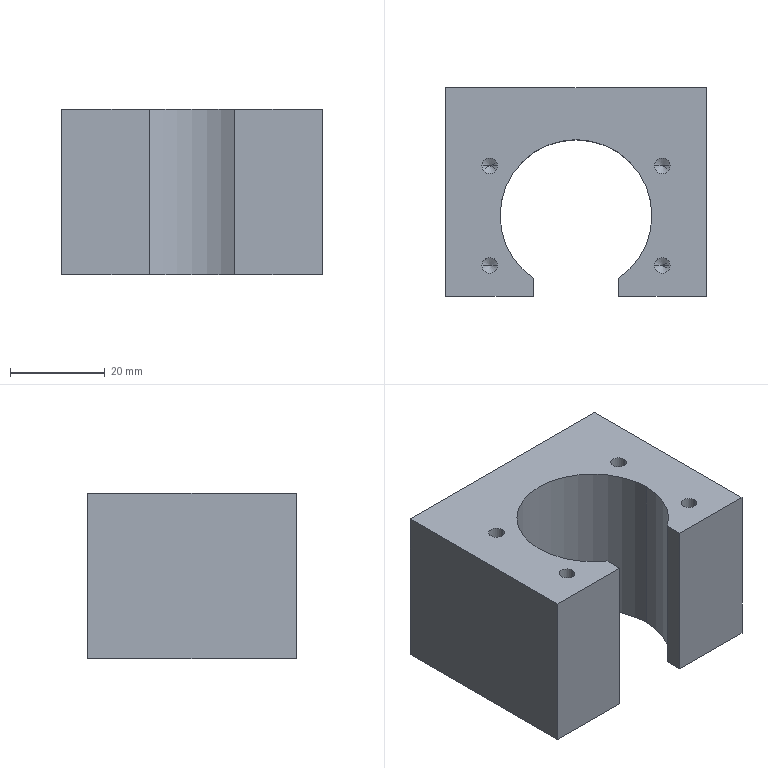Part | SolidWorks | features HoleWzd 2, 3DProfileFeature 1, Extrusion 1 | 1 solid | 52 faces | box 55 x 44 x 35 mm | volume 54034 mm3 | cone 24 | cylinder 19 | plane 9 | commonest cylinder face diameters 3.3 x8 5 x8 32 x3
STEP:
#1=CARTESIAN_POINT('',(-20.5,26.475,8.));
#2=VERTEX_POINT('',#1);
#3=CARTESIAN_POINT('',(-20.5,26.475,13.));
#4=VERTEX_POINT('',#3);
#5=CARTESIAN_POINT('',(-20.5,26.475,10.5));
#6=DIRECTION('',(0.,1.,0.));
#7=DIRECTION('',(0.,0.,1.));
#8=AXIS2_PLACEMENT_3D('',#5,#6,#7);
#9=CIRCLE('',#8,2.5);
#10=EDGE_CURVE('',#2,#4,#9,.T.);
#11=ORIENTED_EDGE('',*,*,#10,.F.);
#12=CARTESIAN_POINT('',(-20.5,27.,7.475));
#13=VERTEX_POINT('',#12);
#14=CARTESIAN_POINT('',(-20.5,27.,7.475));
#15=DIRECTION('',(0.,0.7071,-0.7071));
#16=VECTOR('',#15,1000.);
#17=LINE('',#14,#16);
#18=EDGE_CURVE('',#2,#13,#17,.T.);
#19=ORIENTED_EDGE('',*,*,#18,.T.);
#20=CARTESIAN_POINT('',(-20.5,27.,13.525));
#21=VERTEX_POINT('',#20);
#22=CARTESIAN_POINT('',(-20.5,27.,10.5));
#23=DIRECTION('',(0.,1.,0.));
#24=DIRECTION('',(0.,0.,1.));
#25=AXIS2_PLACEMENT_3D('',#22,#23,#24);
#26=CIRCLE('',#25,3.025);
#27=EDGE_CURVE('',#13,#21,#26,.T.);
#28=ORIENTED_EDGE('',*,*,#27,.T.);
#29=CARTESIAN_POINT('',(-20.5,27.,13.525));
#30=DIRECTION('',(0.,0.7071,0.7071));
#31=VECTOR('',#30,1000.);
#32=LINE('',#29,#31);
#33=EDGE_CURVE('',#4,#21,#32,.T.);
#34=ORIENTED_EDGE('',*,*,#33,.F.);
#35=EDGE_LOOP('',(#11,#19,#28,#34));
#36=FACE_OUTER_BOUND('',#35,.T.);
#37=CARTESIAN_POINT('',(-20.5,27.,10.5));
#38=DIRECTION('',(0.,1.,0.));
#39=DIRECTION('',(0.,0.,1.));
#40=AXIS2_PLACEMENT_3D('',#37,#38,#39);
#41=CONICAL_SURFACE('',#40,3.025,0.7854);
#42=ADVANCED_FACE('',(#36),#41,.F.);
#43=CARTESIAN_POINT('',(-20.5,15.,8.));
#44=VERTEX_POINT('',#43);
#45=CARTESIAN_POINT('',(-20.5,15.,13.));
#46=VERTEX_POINT('',#45);
#47=CARTESIAN_POINT('',(-20.5,15.,10.5));
#48=DIRECTION('',(0.,1.,0.));
#49=DIRECTION('',(0.,0.,1.));
#50=AXIS2_PLACEMENT_3D('',#47,#48,#49);
#51=CIRCLE('',#50,2.5);
#52=EDGE_CURVE('',#44,#46,#51,.T.);
#53=ORIENTED_EDGE('',*,*,#52,.F.);
#54=CARTESIAN_POINT('',(-20.5,27.,8.));
#55=DIRECTION('',(0.,1.,0.));
#56=VECTOR('',#55,1000.);
#57=LINE('',#54,#56);
#58=EDGE_CURVE('',#44,#2,#57,.T.);
#59=ORIENTED_EDGE('',*,*,#58,.T.);
#60=ORIENTED_EDGE('',*,*,#10,.T.);
#61=CARTESIAN_POINT('',(-20.5,27.,13.));
#62=DIRECTION('',(0.,1.,0.));
#63=VECTOR('',#62,1000.);
#64=LINE('',#61,#63);
#65=EDGE_CURVE('',#46,#4,#64,.T.);
#66=ORIENTED_EDGE('',*,*,#65,.F.);
#67=EDGE_LOOP('',(#53,#59,#60,#66));
#68=FACE_OUTER_BOUND('',#67,.T.);
#69=CARTESIAN_POINT('',(-20.5,27.,10.5));
#70=DIRECTION('',(0.,1.,0.));
#71=DIRECTION('',(0.,0.,1.));
#72=AXIS2_PLACEMENT_3D('',#69,#70,#71);
#73=CYLINDRICAL_SURFACE('',#72,2.5);
#74=ADVANCED_FACE('',(#68),#73,.F.);
#75=CARTESIAN_POINT('',(-20.5,13.498,10.5));
#76=VERTEX_POINT('',#75);
#77=CARTESIAN_POINT('',(-20.5,15.,13.));
#78=DIRECTION('',(0.,0.515,0.8572));
#79=VECTOR('',#78,1000.);
#80=LINE('',#77,#79);
#81=EDGE_CURVE('',#76,#46,#80,.T.);
#82=ORIENTED_EDGE('',*,*,#81,.F.);
#83=CARTESIAN_POINT('',(-20.5,15.,8.));
#84=DIRECTION('',(0.,0.515,-0.8572));
#85=VECTOR('',#84,1000.);
#86=LINE('',#83,#85);
#87=EDGE_CURVE('',#76,#44,#86,.T.);
#88=ORIENTED_EDGE('',*,*,#87,.T.);
#89=ORIENTED_EDGE('',*,*,#52,.T.);
#90=EDGE_LOOP('',(#82,#88,#89));
#91=FACE_OUTER_BOUND('',#90,.T.);
#92=CARTESIAN_POINT('',(-20.5,15.,10.5));
#93=DIRECTION('',(0.,1.,0.));
#94=DIRECTION('',(0.,0.,1.));
#95=AXIS2_PLACEMENT_3D('',#92,#93,#94);
#96=CONICAL_SURFACE('',#95,2.5,1.03);
#97=ADVANCED_FACE('',(#91),#96,.F.);
#98=CARTESIAN_POINT('',(-20.5,26.475,-13.));
#99=VERTEX_POINT('',#98);
#100=CARTESIAN_POINT('',(-20.5,26.475,-8.));
#101=VERTEX_POINT('',#100);
#102=CARTESIAN_POINT('',(-20.5,26.475,-10.5));
#103=DIRECTION('',(0.,1.,0.));
#104=DIRECTION('',(0.,0.,1.));
#105=AXIS2_PLACEMENT_3D('',#102,#103,#104);
#106=CIRCLE('',#105,2.5);
#107=EDGE_CURVE('',#99,#101,#106,.T.);
#108=ORIENTED_EDGE('',*,*,#107,.F.);
#109=CARTESIAN_POINT('',(-20.5,27.,-13.525));
#110=VERTEX_POINT('',#109);
#111=CARTESIAN_POINT('',(-20.5,27.,-13.525));
#112=DIRECTION('',(0.,0.7071,-0.7071));
#113=VECTOR('',#112,1000.);
#114=LINE('',#111,#113);
#115=EDGE_CURVE('',#99,#110,#114,.T.);
#116=ORIENTED_EDGE('',*,*,#115,.T.);
#117=CARTESIAN_POINT('',(-20.5,27.,-7.475));
#118=VERTEX_POINT('',#117);
#119=CARTESIAN_POINT('',(-20.5,27.,-10.5));
#120=DIRECTION('',(0.,1.,0.));
#121=DIRECTION('',(0.,0.,1.));
#122=AXIS2_PLACEMENT_3D('',#119,#120,#121);
#123=CIRCLE('',#122,3.025);
#124=EDGE_CURVE('',#110,#118,#123,.T.);
#125=ORIENTED_EDGE('',*,*,#124,.T.);
#126=CARTESIAN_POINT('',(-20.5,27.,-7.475));
#127=DIRECTION('',(0.,0.7071,0.7071));
#128=VECTOR('',#127,1000.);
#129=LINE('',#126,#128);
#130=EDGE_CURVE('',#101,#118,#129,.T.);
#131=ORIENTED_EDGE('',*,*,#130,.F.);
#132=EDGE_LOOP('',(#108,#116,#125,#131));
#133=FACE_OUTER_BOUND('',#132,.T.);
#134=CARTESIAN_POINT('',(-20.5,27.,-10.5));
#135=DIRECTION('',(0.,1.,0.));
#136=DIRECTION('',(0.,0.,1.));
#137=AXIS2_PLACEMENT_3D('',#134,#135,#136);
#138=CONICAL_SURFACE('',#137,3.025,0.7854);
#139=ADVANCED_FACE('',(#133),#138,.F.);
#140=CARTESIAN_POINT('',(-20.5,15.,-13.));
#141=VERTEX_POINT('',#140);
#142=CARTESIAN_POINT('',(-20.5,15.,-8.));
#143=VERTEX_POINT('',#142);
#144=CARTESIAN_POINT('',(-20.5,15.,-10.5));
#145=DIRECTION('',(0.,1.,0.));
#146=DIRECTION('',(0.,0.,1.));
#147=AXIS2_PLACEMENT_3D('',#144,#145,#146);
#148=CIRCLE('',#147,2.5);
#149=EDGE_CURVE('',#141,#143,#148,.T.);
#150=ORIENTED_EDGE('',*,*,#149,.F.);
#151=CARTESIAN_POINT('',(-20.5,27.,-13.));
#152=DIRECTION('',(0.,1.,0.));
#153=VECTOR('',#152,1000.);
#154=LINE('',#151,#153);
#155=EDGE_CURVE('',#141,#99,#154,.T.);
#156=ORIENTED_EDGE('',*,*,#155,.T.);
#157=ORIENTED_EDGE('',*,*,#107,.T.);
#158=CARTESIAN_POINT('',(-20.5,27.,-8.));
#159=DIRECTION('',(0.,1.,0.));
#160=VECTOR('',#159,1000.);
#161=LINE('',#158,#160);
#162=EDGE_CURVE('',#143,#101,#161,.T.);
#163=ORIENTED_EDGE('',*,*,#162,.F.);
#164=EDGE_LOOP('',(#150,#156,#157,#163));
#165=FACE_OUTER_BOUND('',#164,.T.);
#166=CARTESIAN_POINT('',(-20.5,27.,-10.5));
#167=DIRECTION('',(0.,1.,0.));
#168=DIRECTION('',(0.,0.,1.));
#169=AXIS2_PLACEMENT_3D('',#166,#167,#168);
#170=CYLINDRICAL_SURFACE('',#169,2.5);
#171=ADVANCED_FACE('',(#165),#170,.F.);
#172=CARTESIAN_POINT('',(-20.5,13.498,-10.5));
#173=VERTEX_POINT('',#172);
#174=CARTESIAN_POINT('',(-20.5,15.,-8.));
#175=DIRECTION('',(0.,0.515,0.8572));
#176=VECTOR('',#175,1000.);
#177=LINE('',#174,#176);
#178=EDGE_CURVE('',#173,#143,#177,.T.);
#179=ORIENTED_EDGE('',*,*,#178,.F.);
#180=CARTESIAN_POINT('',(-20.5,15.,-13.));
#181=DIRECTION('',(0.,0.515,-0.8572));
#182=VECTOR('',#181,1000.);
#183=LINE('',#180,#182);
#184=EDGE_CURVE('',#173,#141,#183,.T.);
#185=ORIENTED_EDGE('',*,*,#184,.T.);
#186=ORIENTED_EDGE('',*,*,#149,.T.);
#187=EDGE_LOOP('',(#179,#185,#186));
#188=FACE_OUTER_BOUND('',#187,.T.);
#189=CARTESIAN_POINT('',(-20.5,15.,-10.5));
#190=DIRECTION('',(0.,1.,0.));
#191=DIRECTION('',(0.,0.,1.));
#192=AXIS2_PLACEMENT_3D('',#189,#190,#191);
#193=CONICAL_SURFACE('',#192,2.5,1.03);
#194=ADVANCED_FACE('',(#188),#193,.F.);
#195=CARTESIAN_POINT('',(20.5,26.475,-13.));
#196=VERTEX_POINT('',#195);
#197=CARTESIAN_POINT('',(20.5,26.475,-8.));
#198=VERTEX_POINT('',#197);
#199=CARTESIAN_POINT('',(20.5,26.475,-10.5));
#200=DIRECTION('',(0.,1.,0.));
#201=DIRECTION('',(0.,0.,1.));
#202=AXIS2_PLACEMENT_3D('',#199,#200,#201);
#203=CIRCLE('',#202,2.5);
#204=EDGE_CURVE('',#196,#198,#203,.T.);
#205=ORIENTED_EDGE('',*,*,#204,.F.);
#206=CARTESIAN_POINT('',(20.5,27.,-13.525));
#207=VERTEX_POINT('',#206);
#208=CARTESIAN_POINT('',(20.5,27.,-13.525));
#209=DIRECTION('',(0.,0.7071,-0.7071));
#210=VECTOR('',#209,1000.);
#211=LINE('',#208,#210);
#212=EDGE_CURVE('',#196,#207,#211,.T.);
#213=ORIENTED_EDGE('',*,*,#212,.T.);
#214=CARTESIAN_POINT('',(20.5,27.,-7.475));
#215=VERTEX_POINT('',#214);
#216=CARTESIAN_POINT('',(20.5,27.,-10.5));
#217=DIRECTION('',(0.,1.,0.));
#218=DIRECTION('',(0.,0.,1.));
#219=AXIS2_PLACEMENT_3D('',#216,#217,#218);
#220=CIRCLE('',#219,3.025);
#221=EDGE_CURVE('',#207,#215,#220,.T.);
#222=ORIENTED_EDGE('',*,*,#221,.T.);
#223=CARTESIAN_POINT('',(20.5,27.,-7.475));
#224=DIRECTION('',(0.,0.7071,0.7071));
#225=VECTOR('',#224,1000.);
#226=LINE('',#223,#225);
#227=EDGE_CURVE('',#198,#215,#226,.T.);
#228=ORIENTED_EDGE('',*,*,#227,.F.);
#229=EDGE_LOOP('',(#205,#213,#222,#228));
#230=FACE_OUTER_BOUND('',#229,.T.);
#231=CARTESIAN_POINT('',(20.5,27.,-10.5));
#232=DIRECTION('',(0.,1.,0.));
#233=DIRECTION('',(0.,0.,1.));
#234=AXIS2_PLACEMENT_3D('',#231,#232,#233);
#235=CONICAL_SURFACE('',#234,3.025,0.7854);
#236=ADVANCED_FACE('',(#230),#235,.F.);
#237=CARTESIAN_POINT('',(20.5,15.,-13.));
#238=VERTEX_POINT('',#237);
#239=CARTESIAN_POINT('',(20.5,15.,-8.));
#240=VERTEX_POINT('',#239);
#241=CARTESIAN_POINT('',(20.5,15.,-10.5));
#242=DIRECTION('',(0.,1.,0.));
#243=DIRECTION('',(0.,0.,1.));
#244=AXIS2_PLACEMENT_3D('',#241,#242,#243);
#245=CIRCLE('',#244,2.5);
#246=EDGE_CURVE('',#238,#240,#245,.T.);
#247=ORIENTED_EDGE('',*,*,#246,.F.);
#248=CARTESIAN_POINT('',(20.5,27.,-13.));
#249=DIRECTION('',(0.,1.,0.));
#250=VECTOR('',#249,1000.);
#251=LINE('',#248,#250);
#252=EDGE_CURVE('',#238,#196,#251,.T.);
#253=ORIENTED_EDGE('',*,*,#252,.T.);
#254=ORIENTED_EDGE('',*,*,#204,.T.);
#255=CARTESIAN_POINT('',(20.5,27.,-8.));
#256=DIRECTION('',(0.,1.,0.));
#257=VECTOR('',#256,1000.);
#258=LINE('',#255,#257);
#259=EDGE_CURVE('',#240,#198,#258,.T.);
#260=ORIENTED_EDGE('',*,*,#259,.F.);
#261=EDGE_LOOP('',(#247,#253,#254,#260));
#262=FACE_OUTER_BOUND('',#261,.T.);
#263=CARTESIAN_POINT('',(20.5,27.,-10.5));
#264=DIRECTION('',(0.,1.,0.));
#265=DIRECTION('',(0.,0.,1.));
#266=AXIS2_PLACEMENT_3D('',#263,#264,#265);
#267=CYLINDRICAL_SURFACE('',#266,2.5);
#268=ADVANCED_FACE('',(#262),#267,.F.);
#269=CARTESIAN_POINT('',(20.5,13.498,-10.5));
#270=VERTEX_POINT('',#269);
#271=CARTESIAN_POINT('',(20.5,15.,-8.));
#272=DIRECTION('',(0.,0.515,0.8572));
#273=VECTOR('',#272,1000.);
#274=LINE('',#271,#273);
#275=EDGE_CURVE('',#270,#240,#274,.T.);
#276=ORIENTED_EDGE('',*,*,#275,.F.);
#277=CARTESIAN_POINT('',(20.5,15.,-13.));
#278=DIRECTION('',(0.,0.515,-0.8572));
#279=VECTOR('',#278,1000.);
#280=LINE('',#277,#279);
#281=EDGE_CURVE('',#270,#238,#280,.T.);
#282=ORIENTED_EDGE('',*,*,#281,.T.);
#283=ORIENTED_EDGE('',*,*,#246,.T.);
#284=EDGE_LOOP('',(#276,#282,#283));
#285=FACE_OUTER_BOUND('',#284,.T.);
#286=CARTESIAN_POINT('',(20.5,15.,-10.5));
#287=DIRECTION('',(0.,1.,0.));
#288=DIRECTION('',(0.,0.,1.));
#289=AXIS2_PLACEMENT_3D('',#286,#287,#288);
#290=CONICAL_SURFACE('',#289,2.5,1.03);
#291=ADVANCED_FACE('',(#285),#290,.F.);
#292=CARTESIAN_POINT('',(20.5,26.475,8.));
#293=VERTEX_POINT('',#292);
#294=CARTESIAN_POINT('',(20.5,26.475,13.));
#295=VERTEX_POINT('',#294);
#296=CARTESIAN_POINT('',(20.5,26.475,10.5));
#297=DIRECTION('',(0.,1.,0.));
#298=DIRECTION('',(0.,0.,1.));
#299=AXIS2_PLACEMENT_3D('',#296,#297,#298);
#300=CIRCLE('',#299,2.5);
#301=EDGE_CURVE('',#293,#295,#300,.T.);
#302=ORIENTED_EDGE('',*,*,#301,.F.);
#303=CARTESIAN_POINT('',(20.5,27.,7.475));
#304=VERTEX_POINT('',#303);
#305=CARTESIAN_POINT('',(20.5,27.,7.475));
#306=DIRECTION('',(0.,0.7071,-0.7071));
#307=VECTOR('',#306,1000.);
#308=LINE('',#305,#307);
#309=EDGE_CURVE('',#293,#304,#308,.T.);
#310=ORIENTED_EDGE('',*,*,#309,.T.);
#311=CARTESIAN_POINT('',(20.5,27.,13.525));
#312=VERTEX_POINT('',#311);
#313=CARTESIAN_POINT('',(20.5,27.,10.5));
#314=DIRECTION('',(0.,1.,0.));
#315=DIRECTION('',(0.,0.,1.));
#316=AXIS2_PLACEMENT_3D('',#313,#314,#315);
#317=CIRCLE('',#316,3.025);
#318=EDGE_CURVE('',#304,#312,#317,.T.);
#319=ORIENTED_EDGE('',*,*,#318,.T.);
#320=CARTESIAN_POINT('',(20.5,27.,13.525));
#321=DIRECTION('',(0.,0.7071,0.7071));
#322=VECTOR('',#321,1000.);
#323=LINE('',#320,#322);
#324=EDGE_CURVE('',#295,#312,#323,.T.);
#325=ORIENTED_EDGE('',*,*,#324,.F.);
#326=EDGE_LOOP('',(#302,#310,#319,#325));
#327=FACE_OUTER_BOUND('',#326,.T.);
#328=CARTESIAN_POINT('',(20.5,27.,10.5));
#329=DIRECTION('',(0.,1.,0.));
#330=DIRECTION('',(0.,0.,1.));
#331=AXIS2_PLACEMENT_3D('',#328,#329,#330);
#332=CONICAL_SURFACE('',#331,3.025,0.7854);
#333=ADVANCED_FACE('',(#327),#332,.F.);
#334=CARTESIAN_POINT('',(20.5,15.,8.));
#335=VERTEX_POINT('',#334);
#336=CARTESIAN_POINT('',(20.5,15.,13.));
#337=VERTEX_POINT('',#336);
#338=CARTESIAN_POINT('',(20.5,15.,10.5));
#339=DIRECTION('',(0.,1.,0.));
#340=DIRECTION('',(0.,0.,1.));
#341=AXIS2_PLACEMENT_3D('',#338,#339,#340);
#342=CIRCLE('',#341,2.5);
#343=EDGE_CURVE('',#335,#337,#342,.T.);
#344=ORIENTED_EDGE('',*,*,#343,.F.);
#345=CARTESIAN_POINT('',(20.5,27.,8.));
#346=DIRECTION('',(0.,1.,0.));
#347=VECTOR('',#346,1000.);
#348=LINE('',#345,#347);
#349=EDGE_CURVE('',#335,#293,#348,.T.);
#350=ORIENTED_EDGE('',*,*,#349,.T.);
#351=ORIENTED_EDGE('',*,*,#301,.T.);
#352=CARTESIAN_POINT('',(20.5,27.,13.));
#353=DIRECTION('',(0.,1.,0.));
#354=VECTOR('',#353,1000.);
#355=LINE('',#352,#354);
#356=EDGE_CURVE('',#337,#295,#355,.T.);
#357=ORIENTED_EDGE('',*,*,#356,.F.);
#358=EDGE_LOOP('',(#344,#350,#351,#357));
#359=FACE_OUTER_BOUND('',#358,.T.);
#360=CARTESIAN_POINT('',(20.5,27.,10.5));
#361=DIRECTION('',(0.,1.,0.));
#362=DIRECTION('',(0.,0.,1.));
#363=AXIS2_PLACEMENT_3D('',#360,#361,#362);
#364=CYLINDRICAL_SURFACE('',#363,2.5);
#365=ADVANCED_FACE('',(#359),#364,.F.);
#366=CARTESIAN_POINT('',(20.5,13.498,10.5));
#367=VERTEX_POINT('',#366);
#368=CARTESIAN_POINT('',(20.5,15.,13.));
#369=DIRECTION('',(0.,0.515,0.8572));
#370=VECTOR('',#369,1000.);
#371=LINE('',#368,#370);
#372=EDGE_CURVE('',#367,#337,#371,.T.);
#373=ORIENTED_EDGE('',*,*,#372,.F.);
#374=CARTESIAN_POINT('',(20.5,15.,8.));
#375=DIRECTION('',(0.,0.515,-0.8572));
#376=VECTOR('',#375,1000.);
#377=LINE('',#374,#376);
#378=EDGE_CURVE('',#367,#335,#377,.T.);
#379=ORIENTED_EDGE('',*,*,#378,.T.);
#380=ORIENTED_EDGE('',*,*,#343,.T.);
#381=EDGE_LOOP('',(#373,#379,#380));
#382=FACE_OUTER_BOUND('',#381,.T.);
#383=CARTESIAN_POINT('',(20.5,15.,10.5));
#384=DIRECTION('',(0.,1.,0.));
#385=DIRECTION('',(0.,0.,1.));
#386=AXIS2_PLACEMENT_3D('',#383,#384,#385);
#387=CONICAL_SURFACE('',#386,2.5,1.03);
#388=ADVANCED_FACE('',(#382),#387,.F.);
#389=CARTESIAN_POINT('',(16.537,10.5,8.));
#390=VERTEX_POINT('',#389);
#391=CARTESIAN_POINT('',(19.837,10.5,8.));
#392=VERTEX_POINT('',#391);
#393=CARTESIAN_POINT('',(18.187,10.5,8.));
#394=DIRECTION('',(0.,0.,1.));
#395=DIRECTION('',(1.,0.,0.));
#396=AXIS2_PLACEMENT_3D('',#393,#394,#395);
#397=CIRCLE('',#396,1.65);
#398=EDGE_CURVE('',#390,#392,#397,.T.);
#399=ORIENTED_EDGE('',*,*,#398,.F.);
#400=CARTESIAN_POINT('',(16.537,10.5,17.5));
#401=VERTEX_POINT('',#400);
#402=CARTESIAN_POINT('',(16.537,10.5,17.5));
#403=DIRECTION('',(0.,0.,1.));
#404=VECTOR('',#403,1000.);
#405=LINE('',#402,#404);
#406=EDGE_CURVE('',#390,#401,#405,.T.);
#407=ORIENTED_EDGE('',*,*,#406,.T.);
#408=CARTESIAN_POINT('',(19.837,10.5,17.5));
#409=VERTEX_POINT('',#408);
#410=CARTESIAN_POINT('',(18.187,10.5,17.5));
#411=DIRECTION('',(0.,0.,1.));
#412=DIRECTION('',(1.,0.,0.));
#413=AXIS2_PLACEMENT_3D('',#410,#411,#412);
#414=CIRCLE('',#413,1.65);
#415=EDGE_CURVE('',#401,#409,#414,.T.);
#416=ORIENTED_EDGE('',*,*,#415,.T.);
#417=CARTESIAN_POINT('',(19.837,10.5,17.5));
#418=DIRECTION('',(0.,0.,1.));
#419=VECTOR('',#418,1000.);
#420=LINE('',#417,#419);
#421=EDGE_CURVE('',#392,#409,#420,.T.);
#422=ORIENTED_EDGE('',*,*,#421,.F.);
#423=EDGE_LOOP('',(#399,#407,#416,#422));
#424=FACE_OUTER_BOUND('',#423,.T.);
#425=CARTESIAN_POINT('',(18.187,10.5,17.5));
#426=DIRECTION('',(0.,0.,1.));
#427=DIRECTION('',(1.,0.,0.));
#428=AXIS2_PLACEMENT_3D('',#425,#426,#427);
#429=CYLINDRICAL_SURFACE('',#428,1.65);
#430=ADVANCED_FACE('',(#424),#429,.F.);
#431=CARTESIAN_POINT('',(18.187,10.5,7.009));
#432=VERTEX_POINT('',#431);
#433=CARTESIAN_POINT('',(19.837,10.5,8.));
#434=DIRECTION('',(0.8572,0.,0.515));
#435=VECTOR('',#434,1000.);
#436=LINE('',#433,#435);
#437=EDGE_CURVE('',#432,#392,#436,.T.);
#438=ORIENTED_EDGE('',*,*,#437,.F.);
#439=CARTESIAN_POINT('',(16.537,10.5,8.));
#440=DIRECTION('',(-0.8572,0.,0.515));
#441=VECTOR('',#440,1000.);
#442=LINE('',#439,#441);
#443=EDGE_CURVE('',#432,#390,#442,.T.);
#444=ORIENTED_EDGE('',*,*,#443,.T.);
#445=ORIENTED_EDGE('',*,*,#398,.T.);
#446=EDGE_LOOP('',(#438,#444,#445));
#447=FACE_OUTER_BOUND('',#446,.T.);
#448=CARTESIAN_POINT('',(18.187,10.5,8.));
#449=DIRECTION('',(0.,0.,1.));
#450=DIRECTION('',(1.,0.,0.));
#451=AXIS2_PLACEMENT_3D('',#448,#449,#450);
#452=CONICAL_SURFACE('',#451,1.65,1.03);
#453=ADVANCED_FACE('',(#447),#452,.F.);
#454=CARTESIAN_POINT('',(16.537,-10.5,8.));
#455=VERTEX_POINT('',#454);
#456=CARTESIAN_POINT('',(19.837,-10.5,8.));
#457=VERTEX_POINT('',#456);
#458=CARTESIAN_POINT('',(18.187,-10.5,8.));
#459=DIRECTION('',(0.,0.,1.));
#460=DIRECTION('',(1.,0.,0.));
#461=AXIS2_PLACEMENT_3D('',#458,#459,#460);
#462=CIRCLE('',#461,1.65);
#463=EDGE_CURVE('',#455,#457,#462,.T.);
#464=ORIENTED_EDGE('',*,*,#463,.F.);
#465=CARTESIAN_POINT('',(16.537,-10.5,17.5));
#466=VERTEX_POINT('',#465);
#467=CARTESIAN_POINT('',(16.537,-10.5,17.5));
#468=DIRECTION('',(0.,0.,1.));
#469=VECTOR('',#468,1000.);
#470=LINE('',#467,#469);
#471=EDGE_CURVE('',#455,#466,#470,.T.);
#472=ORIENTED_EDGE('',*,*,#471,.T.);
#473=CARTESIAN_POINT('',(19.837,-10.5,17.5));
#474=VERTEX_POINT('',#473);
#475=CARTESIAN_POINT('',(18.187,-10.5,17.5));
#476=DIRECTION('',(0.,0.,1.));
#477=DIRECTION('',(1.,0.,0.));
#478=AXIS2_PLACEMENT_3D('',#475,#476,#477);
#479=CIRCLE('',#478,1.65);
#480=EDGE_CURVE('',#466,#474,#479,.T.);
#481=ORIENTED_EDGE('',*,*,#480,.T.);
#482=CARTESIAN_POINT('',(19.837,-10.5,17.5));
#483=DIRECTION('',(0.,0.,1.));
#484=VECTOR('',#483,1000.);
#485=LINE('',#482,#484);
#486=EDGE_CURVE('',#457,#474,#485,.T.);
#487=ORIENTED_EDGE('',*,*,#486,.F.);
#488=EDGE_LOOP('',(#464,#472,#481,#487));
#489=FACE_OUTER_BOUND('',#488,.T.);
#490=CARTESIAN_POINT('',(18.187,-10.5,17.5));
#491=DIRECTION('',(0.,0.,1.));
#492=DIRECTION('',(1.,0.,0.));
#493=AXIS2_PLACEMENT_3D('',#490,#491,#492);
#494=CYLINDRICAL_SURFACE('',#493,1.65);
#495=ADVANCED_FACE('',(#489),#494,.F.);
#496=CARTESIAN_POINT('',(18.187,-10.5,7.009));
#497=VERTEX_POINT('',#496);
#498=CARTESIAN_POINT('',(19.837,-10.5,8.));
#499=DIRECTION('',(0.8572,0.,0.515));
#500=VECTOR('',#499,1000.);
#501=LINE('',#498,#500);
#502=EDGE_CURVE('',#497,#457,#501,.T.);
#503=ORIENTED_EDGE('',*,*,#502,.F.);
#504=CARTESIAN_POINT('',(16.537,-10.5,8.));
#505=DIRECTION('',(-0.8572,0.,0.515));
#506=VECTOR('',#505,1000.);
#507=LINE('',#504,#506);
#508=EDGE_CURVE('',#497,#455,#507,.T.);
#509=ORIENTED_EDGE('',*,*,#508,.T.);
#510=ORIENTED_EDGE('',*,*,#463,.T.);
#511=EDGE_LOOP('',(#503,#509,#510));
#512=FACE_OUTER_BOUND('',#511,.T.);
#513=CARTESIAN_POINT('',(18.187,-10.5,8.));
#514=DIRECTION('',(0.,0.,1.));
#515=DIRECTION('',(1.,0.,0.));
#516=AXIS2_PLACEMENT_3D('',#513,#514,#515);
#517=CONICAL_SURFACE('',#516,1.65,1.03);
#518=ADVANCED_FACE('',(#512),#517,.F.);
#519=CARTESIAN_POINT('',(-19.837,-10.5,8.));
#520=VERTEX_POINT('',#519);
#521=CARTESIAN_POINT('',(-16.537,-10.5,8.));
#522=VERTEX_POINT('',#521);
#523=CARTESIAN_POINT('',(-18.187,-10.5,8.));
#524=DIRECTION('',(0.,0.,1.));
#525=DIRECTION('',(1.,0.,0.));
#526=AXIS2_PLACEMENT_3D('',#523,#524,#525);
#527=CIRCLE('',#526,1.65);
#528=EDGE_CURVE('',#520,#522,#527,.T.);
#529=ORIENTED_EDGE('',*,*,#528,.F.);
#530=CARTESIAN_POINT('',(-19.837,-10.5,17.5));
#531=VERTEX_POINT('',#530);
#532=CARTESIAN_POINT('',(-19.837,-10.5,17.5));
#533=DIRECTION('',(0.,0.,1.));
#534=VECTOR('',#533,1000.);
#535=LINE('',#532,#534);
#536=EDGE_CURVE('',#520,#531,#535,.T.);
#537=ORIENTED_EDGE('',*,*,#536,.T.);
#538=CARTESIAN_POINT('',(-16.537,-10.5,17.5));
#539=VERTEX_POINT('',#538);
#540=CARTESIAN_POINT('',(-18.187,-10.5,17.5));
#541=DIRECTION('',(0.,0.,1.));
#542=DIRECTION('',(1.,0.,0.));
#543=AXIS2_PLACEMENT_3D('',#540,#541,#542);
#544=CIRCLE('',#543,1.65);
#545=EDGE_CURVE('',#531,#539,#544,.T.);
#546=ORIENTED_EDGE('',*,*,#545,.T.);
#547=CARTESIAN_POINT('',(-16.537,-10.5,17.5));
#548=DIRECTION('',(0.,0.,1.));
#549=VECTOR('',#548,1000.);
#550=LINE('',#547,#549);
#551=EDGE_CURVE('',#522,#539,#550,.T.);
#552=ORIENTED_EDGE('',*,*,#551,.F.);
#553=EDGE_LOOP('',(#529,#537,#546,#552));
#554=FACE_OUTER_BOUND('',#553,.T.);
#555=CARTESIAN_POINT('',(-18.187,-10.5,17.5));
#556=DIRECTION('',(0.,0.,1.));
#557=DIRECTION('',(1.,0.,0.));
#558=AXIS2_PLACEMENT_3D('',#555,#556,#557);
#559=CYLINDRICAL_SURFACE('',#558,1.65);
#560=ADVANCED_FACE('',(#554),#559,.F.);
#561=CARTESIAN_POINT('',(-18.187,-10.5,7.009));
#562=VERTEX_POINT('',#561);
#563=CARTESIAN_POINT('',(-16.537,-10.5,8.));
#564=DIRECTION('',(0.8572,0.,0.515));
#565=VECTOR('',#564,1000.);
#566=LINE('',#563,#565);
#567=EDGE_CURVE('',#562,#522,#566,.T.);
#568=ORIENTED_EDGE('',*,*,#567,.F.);
#569=CARTESIAN_POINT('',(-19.837,-10.5,8.));
#570=DIRECTION('',(-0.8572,0.,0.515));
#571=VECTOR('',#570,1000.);
#572=LINE('',#569,#571);
#573=EDGE_CURVE('',#562,#520,#572,.T.);
#574=ORIENTED_EDGE('',*,*,#573,.T.);
#575=ORIENTED_EDGE('',*,*,#528,.T.);
#576=EDGE_LOOP('',(#568,#574,#575));
#577=FACE_OUTER_BOUND('',#576,.T.);
#578=CARTESIAN_POINT('',(-18.187,-10.5,8.));
#579=DIRECTION('',(0.,0.,1.));
#580=DIRECTION('',(1.,0.,0.));
#581=AXIS2_PLACEMENT_3D('',#578,#579,#580);
#582=CONICAL_SURFACE('',#581,1.65,1.03);
#583=ADVANCED_FACE('',(#577),#582,.F.);
#584=CARTESIAN_POINT('',(-19.837,10.5,8.));
#585=VERTEX_POINT('',#584);
#586=CARTESIAN_POINT('',(-16.537,10.5,8.));
#587=VERTEX_POINT('',#586);
#588=CARTESIAN_POINT('',(-18.187,10.5,8.));
#589=DIRECTION('',(0.,0.,1.));
#590=DIRECTION('',(1.,0.,0.));
#591=AXIS2_PLACEMENT_3D('',#588,#589,#590);
#592=CIRCLE('',#591,1.65);
#593=EDGE_CURVE('',#585,#587,#592,.T.);
#594=ORIENTED_EDGE('',*,*,#593,.F.);
#595=CARTESIAN_POINT('',(-19.837,10.5,17.5));
#596=VERTEX_POINT('',#595);
#597=CARTESIAN_POINT('',(-19.837,10.5,17.5));
#598=DIRECTION('',(0.,0.,1.));
#599=VECTOR('',#598,1000.);
#600=LINE('',#597,#599);
#601=EDGE_CURVE('',#585,#596,#600,.T.);
#602=ORIENTED_EDGE('',*,*,#601,.T.);
#603=CARTESIAN_POINT('',(-16.537,10.5,17.5));
#604=VERTEX_POINT('',#603);
#605=CARTESIAN_POINT('',(-18.187,10.5,17.5));
#606=DIRECTION('',(0.,0.,1.));
#607=DIRECTION('',(1.,0.,0.));
#608=AXIS2_PLACEMENT_3D('',#605,#606,#607);
#609=CIRCLE('',#608,1.65);
#610=EDGE_CURVE('',#596,#604,#609,.T.);
#611=ORIENTED_EDGE('',*,*,#610,.T.);
#612=CARTESIAN_POINT('',(-16.537,10.5,17.5));
#613=DIRECTION('',(0.,0.,1.));
#614=VECTOR('',#613,1000.);
#615=LINE('',#612,#614);
#616=EDGE_CURVE('',#587,#604,#615,.T.);
#617=ORIENTED_EDGE('',*,*,#616,.F.);
#618=EDGE_LOOP('',(#594,#602,#611,#617));
#619=FACE_OUTER_BOUND('',#618,.T.);
#620=CARTESIAN_POINT('',(-18.187,10.5,17.5));
#621=DIRECTION('',(0.,0.,1.));
#622=DIRECTION('',(1.,0.,0.));
#623=AXIS2_PLACEMENT_3D('',#620,#621,#622);
#624=CYLINDRICAL_SURFACE('',#623,1.65);
#625=ADVANCED_FACE('',(#619),#624,.F.);
#626=CARTESIAN_POINT('',(-18.187,10.5,7.009));
#627=VERTEX_POINT('',#626);
#628=CARTESIAN_POINT('',(-16.537,10.5,8.));
#629=DIRECTION('',(0.8572,0.,0.515));
#630=VECTOR('',#629,1000.);
#631=LINE('',#628,#630);
#632=EDGE_CURVE('',#627,#587,#631,.T.);
#633=ORIENTED_EDGE('',*,*,#632,.F.);
#634=CARTESIAN_POINT('',(-19.837,10.5,8.));
#635=DIRECTION('',(-0.8572,0.,0.515));
#636=VECTOR('',#635,1000.);
#637=LINE('',#634,#636);
#638=EDGE_CURVE('',#627,#585,#637,.T.);
#639=ORIENTED_EDGE('',*,*,#638,.T.);
#640=ORIENTED_EDGE('',*,*,#593,.T.);
#641=EDGE_LOOP('',(#633,#639,#640));
#642=FACE_OUTER_BOUND('',#641,.T.);
#643=CARTESIAN_POINT('',(-18.187,10.5,8.));
#644=DIRECTION('',(0.,0.,1.));
#645=DIRECTION('',(1.,0.,0.));
#646=AXIS2_PLACEMENT_3D('',#643,#644,#645);
#647=CONICAL_SURFACE('',#646,1.65,1.03);
#648=ADVANCED_FACE('',(#642),#647,.F.);
#649=CARTESIAN_POINT('',(16.,0.,17.5));
#650=VERTEX_POINT('',#649);
#651=CARTESIAN_POINT('',(9.,-13.229,17.5));
#652=VERTEX_POINT('',#651);
#653=CARTESIAN_POINT('',(0.,0.,17.5));
#654=DIRECTION('',(0.,0.,-1.));
#655=DIRECTION('',(1.,0.,0.));
#656=AXIS2_PLACEMENT_3D('',#653,#654,#655);
#657=CIRCLE('',#656,16.);
#658=EDGE_CURVE('',#650,#652,#657,.T.);
#659=ORIENTED_EDGE('',*,*,#658,.F.);
#660=CARTESIAN_POINT('',(16.,0.,-17.5));
#661=VERTEX_POINT('',#660);
#662=CARTESIAN_POINT('',(16.,0.,17.5));
#663=DIRECTION('',(0.,0.,-1.));
#664=VECTOR('',#663,1000.);
#665=LINE('',#662,#664);
#666=EDGE_CURVE('',#650,#661,#665,.T.);
#667=ORIENTED_EDGE('',*,*,#666,.T.);
#668=CARTESIAN_POINT('',(9.,-13.229,-17.5));
#669=VERTEX_POINT('',#668);
#670=CARTESIAN_POINT('',(0.,0.,-17.5));
#671=DIRECTION('',(0.,0.,-1.));
#672=DIRECTION('',(1.,0.,0.));
#673=AXIS2_PLACEMENT_3D('',#670,#671,#672);
#674=CIRCLE('',#673,16.);
#675=EDGE_CURVE('',#661,#669,#674,.T.);
#676=ORIENTED_EDGE('',*,*,#675,.T.);
#677=CARTESIAN_POINT('',(9.,-13.229,17.5));
#678=DIRECTION('',(0.,0.,-1.));
#679=VECTOR('',#678,1000.);
#680=LINE('',#677,#679);
#681=EDGE_CURVE('',#652,#669,#680,.T.);
#682=ORIENTED_EDGE('',*,*,#681,.F.);
#683=EDGE_LOOP('',(#659,#667,#676,#682));
#684=FACE_OUTER_BOUND('',#683,.T.);
#685=CARTESIAN_POINT('',(0.,0.,17.5));
#686=DIRECTION('',(0.,0.,-1.));
#687=DIRECTION('',(-1.,0.,0.));
#688=AXIS2_PLACEMENT_3D('',#685,#686,#687);
#689=CYLINDRICAL_SURFACE('',#688,16.);
#690=ADVANCED_FACE('',(#684),#689,.F.);
#691=ORIENTED_EDGE('',*,*,#666,.F.);
#692=CARTESIAN_POINT('',(-16.,0.,17.5));
#693=VERTEX_POINT('',#692);
#694=CARTESIAN_POINT('',(0.,0.,17.5));
#695=DIRECTION('',(0.,0.,-1.));
#696=DIRECTION('',(1.,0.,0.));
#697=AXIS2_PLACEMENT_3D('',#694,#695,#696);
#698=CIRCLE('',#697,16.);
#699=EDGE_CURVE('',#693,#650,#698,.T.);
#700=ORIENTED_EDGE('',*,*,#699,.F.);
#701=CARTESIAN_POINT('',(-16.,0.,-17.5));
#702=VERTEX_POINT('',#701);
#703=CARTESIAN_POINT('',(-16.,0.,17.5));
#704=DIRECTION('',(0.,0.,-1.));
#705=VECTOR('',#704,1000.);
#706=LINE('',#703,#705);
#707=EDGE_CURVE('',#693,#702,#706,.T.);
#708=ORIENTED_EDGE('',*,*,#707,.T.);
#709=CARTESIAN_POINT('',(0.,0.,-17.5));
#710=DIRECTION('',(0.,0.,-1.));
#711=DIRECTION('',(1.,0.,0.));
#712=AXIS2_PLACEMENT_3D('',#709,#710,#711);
#713=CIRCLE('',#712,16.);
#714=EDGE_CURVE('',#702,#661,#713,.T.);
#715=ORIENTED_EDGE('',*,*,#714,.T.);
#716=EDGE_LOOP('',(#691,#700,#708,#715));
#717=FACE_OUTER_BOUND('',#716,.T.);
#718=CARTESIAN_POINT('',(0.,0.,17.5));
#719=DIRECTION('',(0.,0.,-1.));
#720=DIRECTION('',(-1.,0.,0.));
#721=AXIS2_PLACEMENT_3D('',#718,#719,#720);
#722=CYLINDRICAL_SURFACE('',#721,16.);
#723=ADVANCED_FACE('',(#717),#722,.F.);
#724=CARTESIAN_POINT('',(-27.5,27.,-17.5));
#725=VERTEX_POINT('',#724);
#726=CARTESIAN_POINT('',(-27.5,-17.,-17.5));
#727=VERTEX_POINT('',#726);
#728=CARTESIAN_POINT('',(-27.5,27.,-17.5));
#729=DIRECTION('',(0.,-1.,0.));
#730=VECTOR('',#729,1000.);
#731=LINE('',#728,#730);
#732=EDGE_CURVE('',#725,#727,#731,.T.);
#733=ORIENTED_EDGE('',*,*,#732,.T.);
#734=CARTESIAN_POINT('',(-27.5,-17.,17.5));
#735=VERTEX_POINT('',#734);
#736=CARTESIAN_POINT('',(-27.5,-17.,17.5));
#737=DIRECTION('',(0.,0.,-1.));
#738=VECTOR('',#737,1000.);
#739=LINE('',#736,#738);
#740=EDGE_CURVE('',#735,#727,#739,.T.);
#741=ORIENTED_EDGE('',*,*,#740,.F.);
#742=CARTESIAN_POINT('',(-27.5,27.,17.5));
#743=VERTEX_POINT('',#742);
#744=CARTESIAN_POINT('',(-27.5,27.,17.5));
#745=DIRECTION('',(0.,-1.,0.));
#746=VECTOR('',#745,1000.);
#747=LINE('',#744,#746);
#748=EDGE_CURVE('',#743,#735,#747,.T.);
#749=ORIENTED_EDGE('',*,*,#748,.F.);
#750=CARTESIAN_POINT('',(-27.5,27.,17.5));
#751=DIRECTION('',(0.,0.,-1.));
#752=VECTOR('',#751,1000.);
#753=LINE('',#750,#752);
#754=EDGE_CURVE('',#743,#725,#753,.T.);
#755=ORIENTED_EDGE('',*,*,#754,.T.);
#756=EDGE_LOOP('',(#733,#741,#749,#755));
#757=FACE_OUTER_BOUND('',#756,.T.);
#758=CARTESIAN_POINT('',(-27.5,27.,17.5));
#759=DIRECTION('',(1.,0.,0.));
#760=DIRECTION('',(0.,0.,-1.));
#761=AXIS2_PLACEMENT_3D('',#758,#759,#760);
#762=PLANE('',#761);
#763=ADVANCED_FACE('',(#757),#762,.F.);
#764=CARTESIAN_POINT('',(-9.,-17.,-17.5));
#765=VERTEX_POINT('',#764);
#766=CARTESIAN_POINT('',(-27.5,-17.,-17.5));
#767=DIRECTION('',(1.,0.,0.));
#768=VECTOR('',#767,1000.);
#769=LINE('',#766,#768);
#770=EDGE_CURVE('',#727,#765,#769,.T.);
#771=ORIENTED_EDGE('',*,*,#770,.T.);
#772=CARTESIAN_POINT('',(-9.,-17.,17.5));
#773=VERTEX_POINT('',#772);
#774=CARTESIAN_POINT('',(-9.,-17.,17.5));
#775=DIRECTION('',(0.,0.,-1.));
#776=VECTOR('',#775,1000.);
#777=LINE('',#774,#776);
#778=EDGE_CURVE('',#773,#765,#777,.T.);
#779=ORIENTED_EDGE('',*,*,#778,.F.);
#780=CARTESIAN_POINT('',(-27.5,-17.,17.5));
#781=DIRECTION('',(1.,0.,0.));
#782=VECTOR('',#781,1000.);
#783=LINE('',#780,#782);
#784=EDGE_CURVE('',#735,#773,#783,.T.);
#785=ORIENTED_EDGE('',*,*,#784,.F.);
#786=ORIENTED_EDGE('',*,*,#740,.T.);
#787=EDGE_LOOP('',(#771,#779,#785,#786));
#788=FACE_OUTER_BOUND('',#787,.T.);
#789=CARTESIAN_POINT('',(-27.5,-17.,17.5));
#790=DIRECTION('',(0.,1.,0.));
#791=DIRECTION('',(0.,0.,1.));
#792=AXIS2_PLACEMENT_3D('',#789,#790,#791);
#793=PLANE('',#792);
#794=ADVANCED_FACE('',(#788),#793,.F.);
#795=CARTESIAN_POINT('',(-9.,-13.229,-17.5));
#796=VERTEX_POINT('',#795);
#797=CARTESIAN_POINT('',(-9.,-17.,-17.5));
#798=DIRECTION('',(0.,1.,0.));
#799=VECTOR('',#798,1000.);
#800=LINE('',#797,#799);
#801=EDGE_CURVE('',#765,#796,#800,.T.);
#802=ORIENTED_EDGE('',*,*,#801,.T.);
#803=CARTESIAN_POINT('',(-9.,-13.229,17.5));
#804=VERTEX_POINT('',#803);
#805=CARTESIAN_POINT('',(-9.,-13.229,17.5));
#806=DIRECTION('',(0.,0.,-1.));
#807=VECTOR('',#806,1000.);
#808=LINE('',#805,#807);
#809=EDGE_CURVE('',#804,#796,#808,.T.);
#810=ORIENTED_EDGE('',*,*,#809,.F.);
#811=CARTESIAN_POINT('',(-9.,-17.,17.5));
#812=DIRECTION('',(0.,1.,0.));
#813=VECTOR('',#812,1000.);
#814=LINE('',#811,#813);
#815=EDGE_CURVE('',#773,#804,#814,.T.);
#816=ORIENTED_EDGE('',*,*,#815,.F.);
#817=ORIENTED_EDGE('',*,*,#778,.T.);
#818=EDGE_LOOP('',(#802,#810,#816,#817));
#819=FACE_OUTER_BOUND('',#818,.T.);
#820=CARTESIAN_POINT('',(-9.,-17.,17.5));
#821=DIRECTION('',(-1.,0.,0.));
#822=DIRECTION('',(0.,-1.,0.));
#823=AXIS2_PLACEMENT_3D('',#820,#821,#822);
#824=PLANE('',#823);
#825=ADVANCED_FACE('',(#819),#824,.F.);
#826=ORIENTED_EDGE('',*,*,#707,.F.);
#827=CARTESIAN_POINT('',(0.,0.,17.5));
#828=DIRECTION('',(0.,0.,-1.));
#829=DIRECTION('',(1.,0.,0.));
#830=AXIS2_PLACEMENT_3D('',#827,#828,#829);
#831=CIRCLE('',#830,16.);
#832=EDGE_CURVE('',#804,#693,#831,.T.);
#833=ORIENTED_EDGE('',*,*,#832,.F.);
#834=ORIENTED_EDGE('',*,*,#809,.T.);
#835=CARTESIAN_POINT('',(0.,0.,-17.5));
#836=DIRECTION('',(0.,0.,-1.));
#837=DIRECTION('',(1.,0.,0.));
#838=AXIS2_PLACEMENT_3D('',#835,#836,#837);
#839=CIRCLE('',#838,16.);
#840=EDGE_CURVE('',#796,#702,#839,.T.);
#841=ORIENTED_EDGE('',*,*,#840,.T.);
#842=EDGE_LOOP('',(#826,#833,#834,#841));
#843=FACE_OUTER_BOUND('',#842,.T.);
#844=CARTESIAN_POINT('',(0.,0.,17.5));
#845=DIRECTION('',(0.,0.,-1.));
#846=DIRECTION('',(-1.,0.,0.));
#847=AXIS2_PLACEMENT_3D('',#844,#845,#846);
#848=CYLINDRICAL_SURFACE('',#847,16.);
#849=ADVANCED_FACE('',(#843),#848,.F.);
#850=CARTESIAN_POINT('',(9.,-17.,-17.5));
#851=VERTEX_POINT('',#850);
#852=CARTESIAN_POINT('',(9.,-17.,-17.5));
#853=DIRECTION('',(0.,-1.,0.));
#854=VECTOR('',#853,1000.);
#855=LINE('',#852,#854);
#856=EDGE_CURVE('',#669,#851,#855,.T.);
#857=ORIENTED_EDGE('',*,*,#856,.T.);
#858=CARTESIAN_POINT('',(9.,-17.,17.5));
#859=VERTEX_POINT('',#858);
#860=CARTESIAN_POINT('',(9.,-17.,17.5));
#861=DIRECTION('',(0.,0.,-1.));
#862=VECTOR('',#861,1000.);
#863=LINE('',#860,#862);
#864=EDGE_CURVE('',#859,#851,#863,.T.);
#865=ORIENTED_EDGE('',*,*,#864,.F.);
#866=CARTESIAN_POINT('',(9.,-17.,17.5));
#867=DIRECTION('',(0.,-1.,0.));
#868=VECTOR('',#867,1000.);
#869=LINE('',#866,#868);
#870=EDGE_CURVE('',#652,#859,#869,.T.);
#871=ORIENTED_EDGE('',*,*,#870,.F.);
#872=ORIENTED_EDGE('',*,*,#681,.T.);
#873=EDGE_LOOP('',(#857,#865,#871,#872));
#874=FACE_OUTER_BOUND('',#873,.T.);
#875=CARTESIAN_POINT('',(9.,-17.,17.5));
#876=DIRECTION('',(1.,0.,0.));
#877=DIRECTION('',(0.,0.,-1.));
#878=AXIS2_PLACEMENT_3D('',#875,#876,#877);
#879=PLANE('',#878);
#880=ADVANCED_FACE('',(#874),#879,.F.);
#881=CARTESIAN_POINT('',(27.5,-17.,-17.5));
#882=VERTEX_POINT('',#881);
#883=CARTESIAN_POINT('',(27.5,-17.,-17.5));
#884=DIRECTION('',(1.,0.,0.));
#885=VECTOR('',#884,1000.);
#886=LINE('',#883,#885);
#887=EDGE_CURVE('',#851,#882,#886,.T.);
#888=ORIENTED_EDGE('',*,*,#887,.T.);
#889=CARTESIAN_POINT('',(27.5,-17.,17.5));
#890=VERTEX_POINT('',#889);
#891=CARTESIAN_POINT('',(27.5,-17.,17.5));
#892=DIRECTION('',(0.,0.,-1.));
#893=VECTOR('',#892,1000.);
#894=LINE('',#891,#893);
#895=EDGE_CURVE('',#890,#882,#894,.T.);
#896=ORIENTED_EDGE('',*,*,#895,.F.);
#897=CARTESIAN_POINT('',(27.5,-17.,17.5));
#898=DIRECTION('',(1.,0.,0.));
#899=VECTOR('',#898,1000.);
#900=LINE('',#897,#899);
#901=EDGE_CURVE('',#859,#890,#900,.T.);
#902=ORIENTED_EDGE('',*,*,#901,.F.);
#903=ORIENTED_EDGE('',*,*,#864,.T.);
#904=EDGE_LOOP('',(#888,#896,#902,#903));
#905=FACE_OUTER_BOUND('',#904,.T.);
#906=CARTESIAN_POINT('',(27.5,-17.,17.5));
#907=DIRECTION('',(0.,1.,0.));
#908=DIRECTION('',(-1.,0.,0.));
#909=AXIS2_PLACEMENT_3D('',#906,#907,#908);
#910=PLANE('',#909);
#911=ADVANCED_FACE('',(#905),#910,.F.);
#912=CARTESIAN_POINT('',(27.5,27.,-17.5));
#913=VERTEX_POINT('',#912);
#914=CARTESIAN_POINT('',(27.5,27.,-17.5));
#915=DIRECTION('',(0.,1.,0.));
#916=VECTOR('',#915,1000.);
#917=LINE('',#914,#916);
#918=EDGE_CURVE('',#882,#913,#917,.T.);
#919=ORIENTED_EDGE('',*,*,#918,.T.);
#920=CARTESIAN_POINT('',(27.5,27.,17.5));
#921=VERTEX_POINT('',#920);
#922=CARTESIAN_POINT('',(27.5,27.,17.5));
#923=DIRECTION('',(0.,0.,-1.));
#924=VECTOR('',#923,1000.);
#925=LINE('',#922,#924);
#926=EDGE_CURVE('',#921,#913,#925,.T.);
#927=ORIENTED_EDGE('',*,*,#926,.F.);
#928=CARTESIAN_POINT('',(27.5,27.,17.5));
#929=DIRECTION('',(0.,1.,0.));
#930=VECTOR('',#929,1000.);
#931=LINE('',#928,#930);
#932=EDGE_CURVE('',#890,#921,#931,.T.);
#933=ORIENTED_EDGE('',*,*,#932,.F.);
#934=ORIENTED_EDGE('',*,*,#895,.T.);
#935=EDGE_LOOP('',(#919,#927,#933,#934));
#936=FACE_OUTER_BOUND('',#935,.T.);
#937=CARTESIAN_POINT('',(27.5,27.,17.5));
#938=DIRECTION('',(-1.,0.,0.));
#939=DIRECTION('',(0.,0.,1.));
#940=AXIS2_PLACEMENT_3D('',#937,#938,#939);
#941=PLANE('',#940);
#942=ADVANCED_FACE('',(#936),#941,.F.);
#943=CARTESIAN_POINT('',(-20.5,27.,10.5));
#944=DIRECTION('',(0.,1.,0.));
#945=DIRECTION('',(0.,0.,1.));
#946=AXIS2_PLACEMENT_3D('',#943,#944,#945);
#947=CIRCLE('',#946,3.025);
#948=EDGE_CURVE('',#21,#13,#947,.T.);
#949=ORIENTED_EDGE('',*,*,#948,.F.);
#950=ORIENTED_EDGE('',*,*,#27,.F.);
#951=EDGE_LOOP('',(#949,#950));
#952=FACE_BOUND('',#951,.T.);
#953=CARTESIAN_POINT('',(-20.5,27.,-10.5));
#954=DIRECTION('',(0.,1.,0.));
#955=DIRECTION('',(0.,0.,1.));
#956=AXIS2_PLACEMENT_3D('',#953,#954,#955);
#957=CIRCLE('',#956,3.025);
#958=EDGE_CURVE('',#118,#110,#957,.T.);
#959=ORIENTED_EDGE('',*,*,#958,.F.);
#960=ORIENTED_EDGE('',*,*,#124,.F.);
#961=EDGE_LOOP('',(#959,#960));
#962=FACE_BOUND('',#961,.T.);
#963=CARTESIAN_POINT('',(20.5,27.,-10.5));
#964=DIRECTION('',(0.,1.,0.));
#965=DIRECTION('',(0.,0.,1.));
#966=AXIS2_PLACEMENT_3D('',#963,#964,#965);
#967=CIRCLE('',#966,3.025);
#968=EDGE_CURVE('',#215,#207,#967,.T.);
#969=ORIENTED_EDGE('',*,*,#968,.F.);
#970=ORIENTED_EDGE('',*,*,#221,.F.);
#971=EDGE_LOOP('',(#969,#970));
#972=FACE_BOUND('',#971,.T.);
#973=CARTESIAN_POINT('',(20.5,27.,10.5));
#974=DIRECTION('',(0.,1.,0.));
#975=DIRECTION('',(0.,0.,1.));
#976=AXIS2_PLACEMENT_3D('',#973,#974,#975);
#977=CIRCLE('',#976,3.025);
#978=EDGE_CURVE('',#312,#304,#977,.T.);
#979=ORIENTED_EDGE('',*,*,#978,.F.);
#980=ORIENTED_EDGE('',*,*,#318,.F.);
#981=EDGE_LOOP('',(#979,#980));
#982=FACE_BOUND('',#981,.T.);
#983=CARTESIAN_POINT('',(-27.5,27.,-17.5));
#984=DIRECTION('',(-1.,0.,0.));
#985=VECTOR('',#984,1000.);
#986=LINE('',#983,#985);
#987=EDGE_CURVE('',#913,#725,#986,.T.);
#988=ORIENTED_EDGE('',*,*,#987,.T.);
#989=ORIENTED_EDGE('',*,*,#754,.F.);
#990=CARTESIAN_POINT('',(-27.5,27.,17.5));
#991=DIRECTION('',(-1.,0.,0.));
#992=VECTOR('',#991,1000.);
#993=LINE('',#990,#992);
#994=EDGE_CURVE('',#921,#743,#993,.T.);
#995=ORIENTED_EDGE('',*,*,#994,.F.);
#996=ORIENTED_EDGE('',*,*,#926,.T.);
#997=EDGE_LOOP('',(#988,#989,#995,#996));
#998=FACE_OUTER_BOUND('',#997,.T.);
#999=CARTESIAN_POINT('',(-27.5,27.,17.5));
#1000=DIRECTION('',(0.,-1.,0.));
#1001=DIRECTION('',(0.,0.,-1.));
#1002=AXIS2_PLACEMENT_3D('',#999,#1000,#1001);
#1003=PLANE('',#1002);
#1004=ADVANCED_FACE('',(#952,#962,#972,#982,#998),#1003,.F.);
#1005=CARTESIAN_POINT('',(18.187,10.5,17.5));
#1006=DIRECTION('',(0.,0.,1.));
#1007=DIRECTION('',(1.,0.,0.));
#1008=AXIS2_PLACEMENT_3D('',#1005,#1006,#1007);
#1009=CIRCLE('',#1008,1.65);
#1010=EDGE_CURVE('',#409,#401,#1009,.T.);
#1011=ORIENTED_EDGE('',*,*,#1010,.F.);
#1012=ORIENTED_EDGE('',*,*,#415,.F.);
#1013=EDGE_LOOP('',(#1011,#1012));
#1014=FACE_BOUND('',#1013,.T.);
#1015=CARTESIAN_POINT('',(18.187,-10.5,17.5));
#1016=DIRECTION('',(0.,0.,1.));
#1017=DIRECTION('',(1.,0.,0.));
#1018=AXIS2_PLACEMENT_3D('',#1015,#1016,#1017);
#1019=CIRCLE('',#1018,1.65);
#1020=EDGE_CURVE('',#474,#466,#1019,.T.);
#1021=ORIENTED_EDGE('',*,*,#1020,.F.);
#1022=ORIENTED_EDGE('',*,*,#480,.F.);
#1023=EDGE_LOOP('',(#1021,#1022));
#1024=FACE_BOUND('',#1023,.T.);
#1025=CARTESIAN_POINT('',(-18.187,-10.5,17.5));
#1026=DIRECTION('',(0.,0.,1.));
#1027=DIRECTION('',(1.,0.,0.));
#1028=AXIS2_PLACEMENT_3D('',#1025,#1026,#1027);
#1029=CIRCLE('',#1028,1.65);
#1030=EDGE_CURVE('',#539,#531,#1029,.T.);
#1031=ORIENTED_EDGE('',*,*,#1030,.F.);
#1032=ORIENTED_EDGE('',*,*,#545,.F.);
#1033=EDGE_LOOP('',(#1031,#1032));
#1034=FACE_BOUND('',#1033,.T.);
#1035=CARTESIAN_POINT('',(-18.187,10.5,17.5));
#1036=DIRECTION('',(0.,0.,1.));
#1037=DIRECTION('',(1.,0.,0.));
#1038=AXIS2_PLACEMENT_3D('',#1035,#1036,#1037);
#1039=CIRCLE('',#1038,1.65);
#1040=EDGE_CURVE('',#604,#596,#1039,.T.);
#1041=ORIENTED_EDGE('',*,*,#1040,.F.);
#1042=ORIENTED_EDGE('',*,*,#610,.F.);
#1043=EDGE_LOOP('',(#1041,#1042));
#1044=FACE_BOUND('',#1043,.T.);
#1045=ORIENTED_EDGE('',*,*,#748,.T.);
#1046=ORIENTED_EDGE('',*,*,#784,.T.);
#1047=ORIENTED_EDGE('',*,*,#815,.T.);
#1048=ORIENTED_EDGE('',*,*,#832,.T.);
#1049=ORIENTED_EDGE('',*,*,#699,.T.);
#1050=ORIENTED_EDGE('',*,*,#658,.T.);
#1051=ORIENTED_EDGE('',*,*,#870,.T.);
#1052=ORIENTED_EDGE('',*,*,#901,.T.);
#1053=ORIENTED_EDGE('',*,*,#932,.T.);
#1054=ORIENTED_EDGE('',*,*,#994,.T.);
#1055=EDGE_LOOP('',(#1045,#1046,#1047,#1048,#1049,#1050,#1051,#1052,#1053,#1054));
#1056=FACE_OUTER_BOUND('',#1055,.T.);
#1057=CARTESIAN_POINT('',(0.,0.,17.5));
#1058=DIRECTION('',(0.,0.,1.));
#1059=DIRECTION('',(1.,0.,0.));
#1060=AXIS2_PLACEMENT_3D('',#1057,#1058,#1059);
#1061=PLANE('',#1060);
#1062=ADVANCED_FACE('',(#1014,#1024,#1034,#1044,#1056),#1061,.T.);
#1063=ORIENTED_EDGE('',*,*,#732,.F.);
#1064=ORIENTED_EDGE('',*,*,#987,.F.);
#1065=ORIENTED_EDGE('',*,*,#918,.F.);
#1066=ORIENTED_EDGE('',*,*,#887,.F.);
#1067=ORIENTED_EDGE('',*,*,#856,.F.);
#1068=ORIENTED_EDGE('',*,*,#675,.F.);
#1069=ORIENTED_EDGE('',*,*,#714,.F.);
#1070=ORIENTED_EDGE('',*,*,#840,.F.);
#1071=ORIENTED_EDGE('',*,*,#801,.F.);
#1072=ORIENTED_EDGE('',*,*,#770,.F.);
#1073=EDGE_LOOP('',(#1063,#1064,#1065,#1066,#1067,#1068,#1069,#1070,#1071,#1072));
#1074=FACE_OUTER_BOUND('',#1073,.T.);
#1075=CARTESIAN_POINT('',(0.,0.,-17.5));
#1076=DIRECTION('',(0.,0.,1.));
#1077=DIRECTION('',(1.,0.,0.));
#1078=AXIS2_PLACEMENT_3D('',#1075,#1076,#1077);
#1079=PLANE('',#1078);
#1080=ADVANCED_FACE('',(#1074),#1079,.F.);
#1081=ORIENTED_EDGE('',*,*,#638,.F.);
#1082=ORIENTED_EDGE('',*,*,#632,.T.);
#1083=CARTESIAN_POINT('',(-18.187,10.5,8.));
#1084=DIRECTION('',(0.,0.,1.));
#1085=DIRECTION('',(1.,0.,0.));
#1086=AXIS2_PLACEMENT_3D('',#1083,#1084,#1085);
#1087=CIRCLE('',#1086,1.65);
#1088=EDGE_CURVE('',#587,#585,#1087,.T.);
#1089=ORIENTED_EDGE('',*,*,#1088,.T.);
#1090=EDGE_LOOP('',(#1081,#1082,#1089));
#1091=FACE_OUTER_BOUND('',#1090,.T.);
#1092=CARTESIAN_POINT('',(-18.187,10.5,8.));
#1093=DIRECTION('',(0.,0.,1.));
#1094=DIRECTION('',(1.,0.,0.));
#1095=AXIS2_PLACEMENT_3D('',#1092,#1093,#1094);
#1096=CONICAL_SURFACE('',#1095,1.65,1.03);
#1097=ADVANCED_FACE('',(#1091),#1096,.F.);
#1098=ORIENTED_EDGE('',*,*,#601,.F.);
#1099=ORIENTED_EDGE('',*,*,#1088,.F.);
#1100=ORIENTED_EDGE('',*,*,#616,.T.);
#1101=ORIENTED_EDGE('',*,*,#1040,.T.);
#1102=EDGE_LOOP('',(#1098,#1099,#1100,#1101));
#1103=FACE_OUTER_BOUND('',#1102,.T.);
#1104=CARTESIAN_POINT('',(-18.187,10.5,17.5));
#1105=DIRECTION('',(0.,0.,1.));
#1106=DIRECTION('',(1.,0.,0.));
#1107=AXIS2_PLACEMENT_3D('',#1104,#1105,#1106);
#1108=CYLINDRICAL_SURFACE('',#1107,1.65);
#1109=ADVANCED_FACE('',(#1103),#1108,.F.);
#1110=ORIENTED_EDGE('',*,*,#573,.F.);
#1111=ORIENTED_EDGE('',*,*,#567,.T.);
#1112=CARTESIAN_POINT('',(-18.187,-10.5,8.));
#1113=DIRECTION('',(0.,0.,1.));
#1114=DIRECTION('',(1.,0.,0.));
#1115=AXIS2_PLACEMENT_3D('',#1112,#1113,#1114);
#1116=CIRCLE('',#1115,1.65);
#1117=EDGE_CURVE('',#522,#520,#1116,.T.);
#1118=ORIENTED_EDGE('',*,*,#1117,.T.);
#1119=EDGE_LOOP('',(#1110,#1111,#1118));
#1120=FACE_OUTER_BOUND('',#1119,.T.);
#1121=CARTESIAN_POINT('',(-18.187,-10.5,8.));
#1122=DIRECTION('',(0.,0.,1.));
#1123=DIRECTION('',(1.,0.,0.));
#1124=AXIS2_PLACEMENT_3D('',#1121,#1122,#1123);
#1125=CONICAL_SURFACE('',#1124,1.65,1.03);
#1126=ADVANCED_FACE('',(#1120),#1125,.F.);
#1127=ORIENTED_EDGE('',*,*,#536,.F.);
#1128=ORIENTED_EDGE('',*,*,#1117,.F.);
#1129=ORIENTED_EDGE('',*,*,#551,.T.);
#1130=ORIENTED_EDGE('',*,*,#1030,.T.);
#1131=EDGE_LOOP('',(#1127,#1128,#1129,#1130));
#1132=FACE_OUTER_BOUND('',#1131,.T.);
#1133=CARTESIAN_POINT('',(-18.187,-10.5,17.5));
#1134=DIRECTION('',(0.,0.,1.));
#1135=DIRECTION('',(1.,0.,0.));
#1136=AXIS2_PLACEMENT_3D('',#1133,#1134,#1135);
#1137=CYLINDRICAL_SURFACE('',#1136,1.65);
#1138=ADVANCED_FACE('',(#1132),#1137,.F.);
#1139=ORIENTED_EDGE('',*,*,#508,.F.);
#1140=ORIENTED_EDGE('',*,*,#502,.T.);
#1141=CARTESIAN_POINT('',(18.187,-10.5,8.));
#1142=DIRECTION('',(0.,0.,1.));
#1143=DIRECTION('',(1.,0.,0.));
#1144=AXIS2_PLACEMENT_3D('',#1141,#1142,#1143);
#1145=CIRCLE('',#1144,1.65);
#1146=EDGE_CURVE('',#457,#455,#1145,.T.);
#1147=ORIENTED_EDGE('',*,*,#1146,.T.);
#1148=EDGE_LOOP('',(#1139,#1140,#1147));
#1149=FACE_OUTER_BOUND('',#1148,.T.);
#1150=CARTESIAN_POINT('',(18.187,-10.5,8.));
#1151=DIRECTION('',(0.,0.,1.));
#1152=DIRECTION('',(1.,0.,0.));
#1153=AXIS2_PLACEMENT_3D('',#1150,#1151,#1152);
#1154=CONICAL_SURFACE('',#1153,1.65,1.03);
#1155=ADVANCED_FACE('',(#1149),#1154,.F.);
#1156=ORIENTED_EDGE('',*,*,#471,.F.);
#1157=ORIENTED_EDGE('',*,*,#1146,.F.);
#1158=ORIENTED_EDGE('',*,*,#486,.T.);
#1159=ORIENTED_EDGE('',*,*,#1020,.T.);
#1160=EDGE_LOOP('',(#1156,#1157,#1158,#1159));
#1161=FACE_OUTER_BOUND('',#1160,.T.);
#1162=CARTESIAN_POINT('',(18.187,-10.5,17.5));
#1163=DIRECTION('',(0.,0.,1.));
#1164=DIRECTION('',(1.,0.,0.));
#1165=AXIS2_PLACEMENT_3D('',#1162,#1163,#1164);
#1166=CYLINDRICAL_SURFACE('',#1165,1.65);
#1167=ADVANCED_FACE('',(#1161),#1166,.F.);
#1168=ORIENTED_EDGE('',*,*,#443,.F.);
#1169=ORIENTED_EDGE('',*,*,#437,.T.);
#1170=CARTESIAN_POINT('',(18.187,10.5,8.));
#1171=DIRECTION('',(0.,0.,1.));
#1172=DIRECTION('',(1.,0.,0.));
#1173=AXIS2_PLACEMENT_3D('',#1170,#1171,#1172);
#1174=CIRCLE('',#1173,1.65);
#1175=EDGE_CURVE('',#392,#390,#1174,.T.);
#1176=ORIENTED_EDGE('',*,*,#1175,.T.);
#1177=EDGE_LOOP('',(#1168,#1169,#1176));
#1178=FACE_OUTER_BOUND('',#1177,.T.);
#1179=CARTESIAN_POINT('',(18.187,10.5,8.));
#1180=DIRECTION('',(0.,0.,1.));
#1181=DIRECTION('',(1.,0.,0.));
#1182=AXIS2_PLACEMENT_3D('',#1179,#1180,#1181);
#1183=CONICAL_SURFACE('',#1182,1.65,1.03);
#1184=ADVANCED_FACE('',(#1178),#1183,.F.);
#1185=ORIENTED_EDGE('',*,*,#406,.F.);
#1186=ORIENTED_EDGE('',*,*,#1175,.F.);
#1187=ORIENTED_EDGE('',*,*,#421,.T.);
#1188=ORIENTED_EDGE('',*,*,#1010,.T.);
#1189=EDGE_LOOP('',(#1185,#1186,#1187,#1188));
#1190=FACE_OUTER_BOUND('',#1189,.T.);
#1191=CARTESIAN_POINT('',(18.187,10.5,17.5));
#1192=DIRECTION('',(0.,0.,1.));
#1193=DIRECTION('',(1.,0.,0.));
#1194=AXIS2_PLACEMENT_3D('',#1191,#1192,#1193);
#1195=CYLINDRICAL_SURFACE('',#1194,1.65);
#1196=ADVANCED_FACE('',(#1190),#1195,.F.);
#1197=ORIENTED_EDGE('',*,*,#378,.F.);
#1198=ORIENTED_EDGE('',*,*,#372,.T.);
#1199=CARTESIAN_POINT('',(20.5,15.,10.5));
#1200=DIRECTION('',(0.,1.,0.));
#1201=DIRECTION('',(0.,0.,1.));
#1202=AXIS2_PLACEMENT_3D('',#1199,#1200,#1201);
#1203=CIRCLE('',#1202,2.5);
#1204=EDGE_CURVE('',#337,#335,#1203,.T.);
#1205=ORIENTED_EDGE('',*,*,#1204,.T.);
#1206=EDGE_LOOP('',(#1197,#1198,#1205));
#1207=FACE_OUTER_BOUND('',#1206,.T.);
#1208=CARTESIAN_POINT('',(20.5,15.,10.5));
#1209=DIRECTION('',(0.,1.,0.));
#1210=DIRECTION('',(0.,0.,1.));
#1211=AXIS2_PLACEMENT_3D('',#1208,#1209,#1210);
#1212=CONICAL_SURFACE('',#1211,2.5,1.03);
#1213=ADVANCED_FACE('',(#1207),#1212,.F.);
#1214=ORIENTED_EDGE('',*,*,#349,.F.);
#1215=ORIENTED_EDGE('',*,*,#1204,.F.);
#1216=ORIENTED_EDGE('',*,*,#356,.T.);
#1217=CARTESIAN_POINT('',(20.5,26.475,10.5));
#1218=DIRECTION('',(0.,1.,0.));
#1219=DIRECTION('',(0.,0.,1.));
#1220=AXIS2_PLACEMENT_3D('',#1217,#1218,#1219);
#1221=CIRCLE('',#1220,2.5);
#1222=EDGE_CURVE('',#295,#293,#1221,.T.);
#1223=ORIENTED_EDGE('',*,*,#1222,.T.);
#1224=EDGE_LOOP('',(#1214,#1215,#1216,#1223));
#1225=FACE_OUTER_BOUND('',#1224,.T.);
#1226=CARTESIAN_POINT('',(20.5,27.,10.5));
#1227=DIRECTION('',(0.,1.,0.));
#1228=DIRECTION('',(0.,0.,1.));
#1229=AXIS2_PLACEMENT_3D('',#1226,#1227,#1228);
#1230=CYLINDRICAL_SURFACE('',#1229,2.5);
#1231=ADVANCED_FACE('',(#1225),#1230,.F.);
#1232=ORIENTED_EDGE('',*,*,#309,.F.);
#1233=ORIENTED_EDGE('',*,*,#1222,.F.);
#1234=ORIENTED_EDGE('',*,*,#324,.T.);
#1235=ORIENTED_EDGE('',*,*,#978,.T.);
#1236=EDGE_LOOP('',(#1232,#1233,#1234,#1235));
#1237=FACE_OUTER_BOUND('',#1236,.T.);
#1238=CARTESIAN_POINT('',(20.5,27.,10.5));
#1239=DIRECTION('',(0.,1.,0.));
#1240=DIRECTION('',(0.,0.,1.));
#1241=AXIS2_PLACEMENT_3D('',#1238,#1239,#1240);
#1242=CONICAL_SURFACE('',#1241,3.025,0.7854);
#1243=ADVANCED_FACE('',(#1237),#1242,.F.);
#1244=ORIENTED_EDGE('',*,*,#281,.F.);
#1245=ORIENTED_EDGE('',*,*,#275,.T.);
#1246=CARTESIAN_POINT('',(20.5,15.,-10.5));
#1247=DIRECTION('',(0.,1.,0.));
#1248=DIRECTION('',(0.,0.,1.));
#1249=AXIS2_PLACEMENT_3D('',#1246,#1247,#1248);
#1250=CIRCLE('',#1249,2.5);
#1251=EDGE_CURVE('',#240,#238,#1250,.T.);
#1252=ORIENTED_EDGE('',*,*,#1251,.T.);
#1253=EDGE_LOOP('',(#1244,#1245,#1252));
#1254=FACE_OUTER_BOUND('',#1253,.T.);
#1255=CARTESIAN_POINT('',(20.5,15.,-10.5));
#1256=DIRECTION('',(0.,1.,0.));
#1257=DIRECTION('',(0.,0.,1.));
#1258=AXIS2_PLACEMENT_3D('',#1255,#1256,#1257);
#1259=CONICAL_SURFACE('',#1258,2.5,1.03);
#1260=ADVANCED_FACE('',(#1254),#1259,.F.);
#1261=ORIENTED_EDGE('',*,*,#252,.F.);
#1262=ORIENTED_EDGE('',*,*,#1251,.F.);
#1263=ORIENTED_EDGE('',*,*,#259,.T.);
#1264=CARTESIAN_POINT('',(20.5,26.475,-10.5));
#1265=DIRECTION('',(0.,1.,0.));
#1266=DIRECTION('',(0.,0.,1.));
#1267=AXIS2_PLACEMENT_3D('',#1264,#1265,#1266);
#1268=CIRCLE('',#1267,2.5);
#1269=EDGE_CURVE('',#198,#196,#1268,.T.);
#1270=ORIENTED_EDGE('',*,*,#1269,.T.);
#1271=EDGE_LOOP('',(#1261,#1262,#1263,#1270));
#1272=FACE_OUTER_BOUND('',#1271,.T.);
#1273=CARTESIAN_POINT('',(20.5,27.,-10.5));
#1274=DIRECTION('',(0.,1.,0.));
#1275=DIRECTION('',(0.,0.,1.));
#1276=AXIS2_PLACEMENT_3D('',#1273,#1274,#1275);
#1277=CYLINDRICAL_SURFACE('',#1276,2.5);
#1278=ADVANCED_FACE('',(#1272),#1277,.F.);
#1279=ORIENTED_EDGE('',*,*,#212,.F.);
#1280=ORIENTED_EDGE('',*,*,#1269,.F.);
#1281=ORIENTED_EDGE('',*,*,#227,.T.);
#1282=ORIENTED_EDGE('',*,*,#968,.T.);
#1283=EDGE_LOOP('',(#1279,#1280,#1281,#1282));
#1284=FACE_OUTER_BOUND('',#1283,.T.);
#1285=CARTESIAN_POINT('',(20.5,27.,-10.5));
#1286=DIRECTION('',(0.,1.,0.));
#1287=DIRECTION('',(0.,0.,1.));
#1288=AXIS2_PLACEMENT_3D('',#1285,#1286,#1287);
#1289=CONICAL_SURFACE('',#1288,3.025,0.7854);
#1290=ADVANCED_FACE('',(#1284),#1289,.F.);
#1291=ORIENTED_EDGE('',*,*,#184,.F.);
#1292=ORIENTED_EDGE('',*,*,#178,.T.);
#1293=CARTESIAN_POINT('',(-20.5,15.,-10.5));
#1294=DIRECTION('',(0.,1.,0.));
#1295=DIRECTION('',(0.,0.,1.));
#1296=AXIS2_PLACEMENT_3D('',#1293,#1294,#1295);
#1297=CIRCLE('',#1296,2.5);
#1298=EDGE_CURVE('',#143,#141,#1297,.T.);
#1299=ORIENTED_EDGE('',*,*,#1298,.T.);
#1300=EDGE_LOOP('',(#1291,#1292,#1299));
#1301=FACE_OUTER_BOUND('',#1300,.T.);
#1302=CARTESIAN_POINT('',(-20.5,15.,-10.5));
#1303=DIRECTION('',(0.,1.,0.));
#1304=DIRECTION('',(0.,0.,1.));
#1305=AXIS2_PLACEMENT_3D('',#1302,#1303,#1304);
#1306=CONICAL_SURFACE('',#1305,2.5,1.03);
#1307=ADVANCED_FACE('',(#1301),#1306,.F.);
#1308=ORIENTED_EDGE('',*,*,#155,.F.);
#1309=ORIENTED_EDGE('',*,*,#1298,.F.);
#1310=ORIENTED_EDGE('',*,*,#162,.T.);
#1311=CARTESIAN_POINT('',(-20.5,26.475,-10.5));
#1312=DIRECTION('',(0.,1.,0.));
#1313=DIRECTION('',(0.,0.,1.));
#1314=AXIS2_PLACEMENT_3D('',#1311,#1312,#1313);
#1315=CIRCLE('',#1314,2.5);
#1316=EDGE_CURVE('',#101,#99,#1315,.T.);
#1317=ORIENTED_EDGE('',*,*,#1316,.T.);
#1318=EDGE_LOOP('',(#1308,#1309,#1310,#1317));
#1319=FACE_OUTER_BOUND('',#1318,.T.);
#1320=CARTESIAN_POINT('',(-20.5,27.,-10.5));
#1321=DIRECTION('',(0.,1.,0.));
#1322=DIRECTION('',(0.,0.,1.));
#1323=AXIS2_PLACEMENT_3D('',#1320,#1321,#1322);
#1324=CYLINDRICAL_SURFACE('',#1323,2.5);
#1325=ADVANCED_FACE('',(#1319),#1324,.F.);
#1326=ORIENTED_EDGE('',*,*,#115,.F.);
#1327=ORIENTED_EDGE('',*,*,#1316,.F.);
#1328=ORIENTED_EDGE('',*,*,#130,.T.);
#1329=ORIENTED_EDGE('',*,*,#958,.T.);
#1330=EDGE_LOOP('',(#1326,#1327,#1328,#1329));
#1331=FACE_OUTER_BOUND('',#1330,.T.);
#1332=CARTESIAN_POINT('',(-20.5,27.,-10.5));
#1333=DIRECTION('',(0.,1.,0.));
#1334=DIRECTION('',(0.,0.,1.));
#1335=AXIS2_PLACEMENT_3D('',#1332,#1333,#1334);
#1336=CONICAL_SURFACE('',#1335,3.025,0.7854);
#1337=ADVANCED_FACE('',(#1331),#1336,.F.);
#1338=ORIENTED_EDGE('',*,*,#87,.F.);
#1339=ORIENTED_EDGE('',*,*,#81,.T.);
#1340=CARTESIAN_POINT('',(-20.5,15.,10.5));
#1341=DIRECTION('',(0.,1.,0.));
#1342=DIRECTION('',(0.,0.,1.));
#1343=AXIS2_PLACEMENT_3D('',#1340,#1341,#1342);
#1344=CIRCLE('',#1343,2.5);
#1345=EDGE_CURVE('',#46,#44,#1344,.T.);
#1346=ORIENTED_EDGE('',*,*,#1345,.T.);
#1347=EDGE_LOOP('',(#1338,#1339,#1346));
#1348=FACE_OUTER_BOUND('',#1347,.T.);
#1349=CARTESIAN_POINT('',(-20.5,15.,10.5));
#1350=DIRECTION('',(0.,1.,0.));
#1351=DIRECTION('',(0.,0.,1.));
#1352=AXIS2_PLACEMENT_3D('',#1349,#1350,#1351);
#1353=CONICAL_SURFACE('',#1352,2.5,1.03);
#1354=ADVANCED_FACE('',(#1348),#1353,.F.);
#1355=ORIENTED_EDGE('',*,*,#58,.F.);
#1356=ORIENTED_EDGE('',*,*,#1345,.F.);
#1357=ORIENTED_EDGE('',*,*,#65,.T.);
#1358=CARTESIAN_POINT('',(-20.5,26.475,10.5));
#1359=DIRECTION('',(0.,1.,0.));
#1360=DIRECTION('',(0.,0.,1.));
#1361=AXIS2_PLACEMENT_3D('',#1358,#1359,#1360);
#1362=CIRCLE('',#1361,2.5);
#1363=EDGE_CURVE('',#4,#2,#1362,.T.);
#1364=ORIENTED_EDGE('',*,*,#1363,.T.);
#1365=EDGE_LOOP('',(#1355,#1356,#1357,#1364));
#1366=FACE_OUTER_BOUND('',#1365,.T.);
#1367=CARTESIAN_POINT('',(-20.5,27.,10.5));
#1368=DIRECTION('',(0.,1.,0.));
#1369=DIRECTION('',(0.,0.,1.));
#1370=AXIS2_PLACEMENT_3D('',#1367,#1368,#1369);
#1371=CYLINDRICAL_SURFACE('',#1370,2.5);
#1372=ADVANCED_FACE('',(#1366),#1371,.F.);
#1373=ORIENTED_EDGE('',*,*,#18,.F.);
#1374=ORIENTED_EDGE('',*,*,#1363,.F.);
#1375=ORIENTED_EDGE('',*,*,#33,.T.);
#1376=ORIENTED_EDGE('',*,*,#948,.T.);
#1377=EDGE_LOOP('',(#1373,#1374,#1375,#1376));
#1378=FACE_OUTER_BOUND('',#1377,.T.);
#1379=CARTESIAN_POINT('',(-20.5,27.,10.5));
#1380=DIRECTION('',(0.,1.,0.));
#1381=DIRECTION('',(0.,0.,1.));
#1382=AXIS2_PLACEMENT_3D('',#1379,#1380,#1381);
#1383=CONICAL_SURFACE('',#1382,3.025,0.7854);
#1384=ADVANCED_FACE('',(#1378),#1383,.F.);
#1385=CLOSED_SHELL('',(#42,#74,#97,#139,#171,#194,#236,#268,#291,#333,#365,#388,#430,#453,#495,#518,#560,#583,#625,#648,#690,#723,#763,#794,#825,#849,#880,#911,#942,#1004,#1062,#1080,#1097,#1109,#1126,#1138,#1155,#1167,#1184,#1196,#1213,#1231,#1243,#1260,#1278,#1290,#1307,#1325,#1337,#1354,#1372,#1384));
#1386=MANIFOLD_SOLID_BREP('',#1385);
#1387=CARTESIAN_POINT('',(0.,0.,0.));
#1388=DIRECTION('',(0.,0.,1.));
#1389=DIRECTION('',(1.,0.,0.));
#1390=AXIS2_PLACEMENT_3D('',#1387,#1388,#1389);
#1391=(LENGTH_UNIT()NAMED_UNIT(*)SI_UNIT(.MILLI.,.METRE.));
#1392=UNCERTAINTY_MEASURE_WITH_UNIT(LENGTH_MEASURE(0.00001),#1391,'','');
#1393=(NAMED_UNIT(*)PLANE_ANGLE_UNIT()SI_UNIT($,.RADIAN.));
#1394=(NAMED_UNIT(*)SI_UNIT($,.STERADIAN.)SOLID_ANGLE_UNIT());
#1395=(GEOMETRIC_REPRESENTATION_CONTEXT(3)GLOBAL_UNCERTAINTY_ASSIGNED_CONTEXT((#1392))GLOBAL_UNIT_ASSIGNED_CONTEXT((#1391,#1393,#1394))REPRESENTATION_CONTEXT('',''));
#1396=ADVANCED_BREP_SHAPE_REPRESENTATION('',(#1386,#1390),#1395);